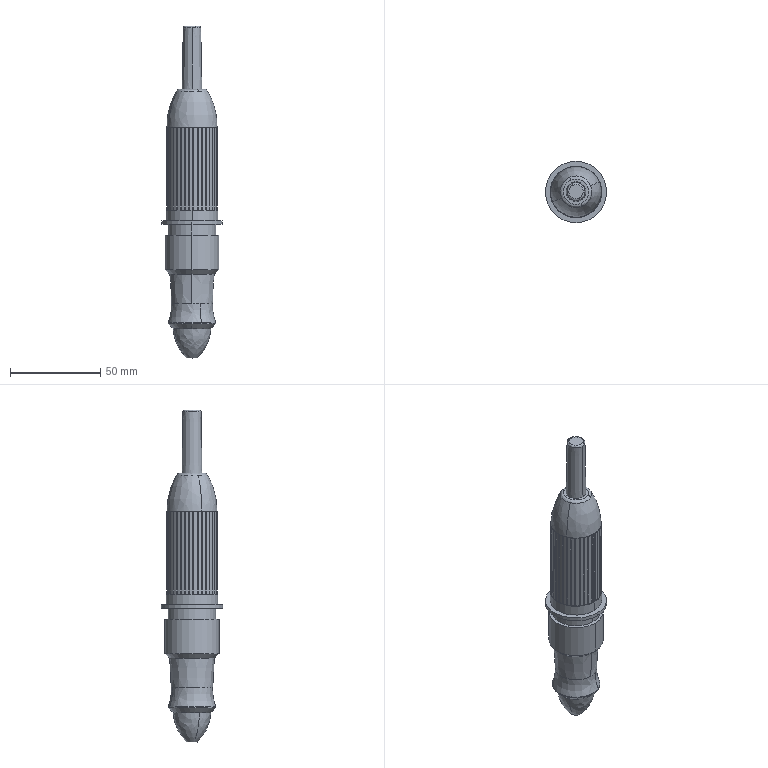Part | SolidWorks | features BaseBody 1 | 1 solid | 151 faces | box 34 x 34 x 184 mm | volume 82006 mm3 | cylinder 90 | plane 43 | spline 10 | cone 8 | commonest cylinder face diameters 1 x43 28 x37 26.5 x4 28.5 x2 30 x2 34 x2